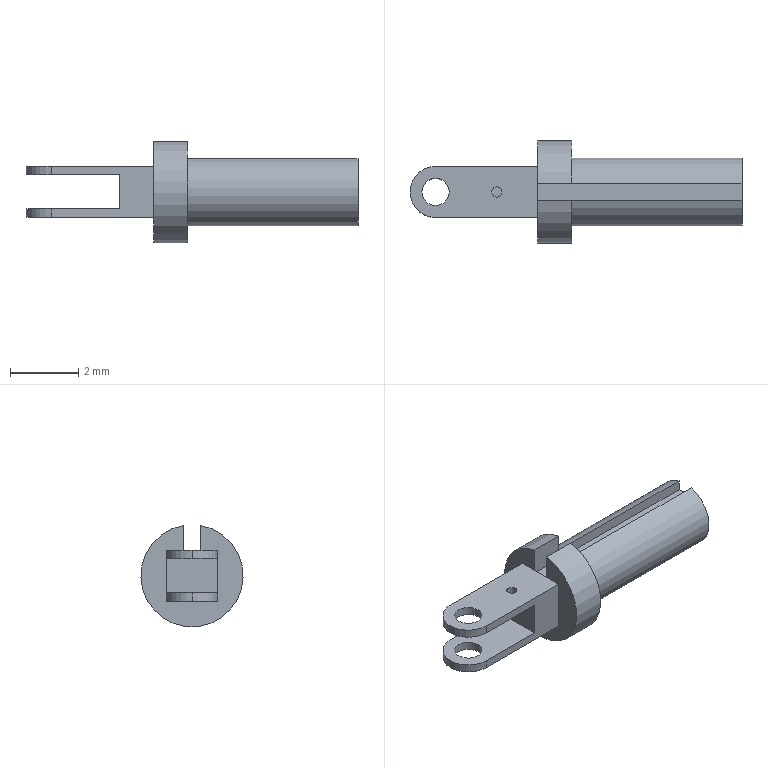Part | SolidWorks | features ICE 5, Revolution 1 | 1 solid | 29 faces | box 9.75 x 3 x 2.979 mm | volume 20.717 mm3 | plane 15 | cylinder 14 | commonest cylinder face diameters 0.8 x4 1.5 x4 0.3 x2 1 x2 2 x1 3 x1
STEP:
#1=CARTESIAN_POINT('',(-1.05,0.,0.5));
#2=VERTEX_POINT('',#1);
#3=CARTESIAN_POINT('',(-1.35,0.,0.5));
#4=VERTEX_POINT('',#3);
#5=CARTESIAN_POINT('',(-1.2,0.,0.5));
#6=DIRECTION('',(0.,0.,-1.));
#7=DIRECTION('',(-1.,0.,0.));
#8=AXIS2_PLACEMENT_3D('',#5,#6,#7);
#9=CIRCLE('',#8,0.15);
#10=EDGE_CURVE('',#2,#4,#9,.T.);
#11=ORIENTED_EDGE('',*,*,#10,.T.);
#12=CARTESIAN_POINT('',(-1.35,0.,0.75));
#13=VERTEX_POINT('',#12);
#14=CARTESIAN_POINT('',(-1.35,0.,-0.25));
#15=DIRECTION('',(0.,0.,1.));
#16=VECTOR('',#15,1000.);
#17=LINE('',#14,#16);
#18=EDGE_CURVE('',#4,#13,#17,.T.);
#19=ORIENTED_EDGE('',*,*,#18,.T.);
#20=CARTESIAN_POINT('',(-1.05,0.,0.75));
#21=VERTEX_POINT('',#20);
#22=CARTESIAN_POINT('',(-1.2,0.,0.75));
#23=DIRECTION('',(0.,0.,1.));
#24=DIRECTION('',(1.,0.,0.));
#25=AXIS2_PLACEMENT_3D('',#22,#23,#24);
#26=CIRCLE('',#25,0.15);
#27=EDGE_CURVE('',#13,#21,#26,.T.);
#28=ORIENTED_EDGE('',*,*,#27,.T.);
#29=CARTESIAN_POINT('',(-1.05,0.,-0.25));
#30=DIRECTION('',(0.,0.,1.));
#31=VECTOR('',#30,1000.);
#32=LINE('',#29,#31);
#33=EDGE_CURVE('',#2,#21,#32,.T.);
#34=ORIENTED_EDGE('',*,*,#33,.F.);
#35=EDGE_LOOP('',(#11,#19,#28,#34));
#36=FACE_OUTER_BOUND('',#35,.T.);
#37=CARTESIAN_POINT('',(-1.2,0.,-0.25));
#38=DIRECTION('',(0.,0.,1.));
#39=DIRECTION('',(1.,0.,0.));
#40=AXIS2_PLACEMENT_3D('',#37,#38,#39);
#41=CYLINDRICAL_SURFACE('',#40,0.15);
#42=ADVANCED_FACE('',(#36),#41,.F.);
#43=CARTESIAN_POINT('',(0.,0.,0.5));
#44=VERTEX_POINT('',#43);
#45=CARTESIAN_POINT('',(0.,0.,-0.5));
#46=VERTEX_POINT('',#45);
#47=CARTESIAN_POINT('',(0.,0.,0.));
#48=DIRECTION('',(1.,0.,0.));
#49=DIRECTION('',(0.,0.,-1.));
#50=AXIS2_PLACEMENT_3D('',#47,#48,#49);
#51=CIRCLE('',#50,0.5);
#52=EDGE_CURVE('',#44,#46,#51,.T.);
#53=ORIENTED_EDGE('',*,*,#52,.F.);
#54=CARTESIAN_POINT('',(6.,0.,0.5));
#55=VERTEX_POINT('',#54);
#56=CARTESIAN_POINT('',(0.,0.,0.5));
#57=DIRECTION('',(1.,0.,0.));
#58=VECTOR('',#57,1000.);
#59=LINE('',#56,#58);
#60=EDGE_CURVE('',#44,#55,#59,.T.);
#61=ORIENTED_EDGE('',*,*,#60,.T.);
#62=CARTESIAN_POINT('',(6.,0.,-0.5));
#63=VERTEX_POINT('',#62);
#64=CARTESIAN_POINT('',(6.,0.,0.));
#65=DIRECTION('',(1.,0.,0.));
#66=DIRECTION('',(0.,0.,-1.));
#67=AXIS2_PLACEMENT_3D('',#64,#65,#66);
#68=CIRCLE('',#67,0.5);
#69=EDGE_CURVE('',#55,#63,#68,.T.);
#70=ORIENTED_EDGE('',*,*,#69,.T.);
#71=CARTESIAN_POINT('',(0.,0.,-0.5));
#72=DIRECTION('',(1.,0.,0.));
#73=VECTOR('',#72,1000.);
#74=LINE('',#71,#73);
#75=EDGE_CURVE('',#46,#63,#74,.T.);
#76=ORIENTED_EDGE('',*,*,#75,.F.);
#77=EDGE_LOOP('',(#53,#61,#70,#76));
#78=FACE_OUTER_BOUND('',#77,.T.);
#79=CARTESIAN_POINT('',(0.,0.,0.));
#80=DIRECTION('',(1.,0.,0.));
#81=DIRECTION('',(0.,0.,-1.));
#82=AXIS2_PLACEMENT_3D('',#79,#80,#81);
#83=CYLINDRICAL_SURFACE('',#82,0.5);
#84=ADVANCED_FACE('',(#78),#83,.F.);
#85=CARTESIAN_POINT('',(-2.6,0.,-0.5));
#86=VERTEX_POINT('',#85);
#87=CARTESIAN_POINT('',(-3.4,0.,-0.5));
#88=VERTEX_POINT('',#87);
#89=CARTESIAN_POINT('',(-3.,0.,-0.5));
#90=DIRECTION('',(0.,0.,-1.));
#91=DIRECTION('',(-1.,0.,0.));
#92=AXIS2_PLACEMENT_3D('',#89,#90,#91);
#93=CIRCLE('',#92,0.4);
#94=EDGE_CURVE('',#86,#88,#93,.T.);
#95=ORIENTED_EDGE('',*,*,#94,.F.);
#96=CARTESIAN_POINT('',(-2.6,0.,-0.75));
#97=VERTEX_POINT('',#96);
#98=CARTESIAN_POINT('',(-2.6,0.,0.75));
#99=DIRECTION('',(0.,0.,-1.));
#100=VECTOR('',#99,1000.);
#101=LINE('',#98,#100);
#102=EDGE_CURVE('',#86,#97,#101,.T.);
#103=ORIENTED_EDGE('',*,*,#102,.T.);
#104=CARTESIAN_POINT('',(-3.4,0.,-0.75));
#105=VERTEX_POINT('',#104);
#106=CARTESIAN_POINT('',(-3.,0.,-0.75));
#107=DIRECTION('',(0.,0.,1.));
#108=DIRECTION('',(1.,0.,0.));
#109=AXIS2_PLACEMENT_3D('',#106,#107,#108);
#110=CIRCLE('',#109,0.4);
#111=EDGE_CURVE('',#105,#97,#110,.T.);
#112=ORIENTED_EDGE('',*,*,#111,.F.);
#113=CARTESIAN_POINT('',(-3.4,0.,0.75));
#114=DIRECTION('',(0.,0.,-1.));
#115=VECTOR('',#114,1000.);
#116=LINE('',#113,#115);
#117=EDGE_CURVE('',#88,#105,#116,.T.);
#118=ORIENTED_EDGE('',*,*,#117,.F.);
#119=EDGE_LOOP('',(#95,#103,#112,#118));
#120=FACE_OUTER_BOUND('',#119,.T.);
#121=CARTESIAN_POINT('',(-3.,0.,0.75));
#122=DIRECTION('',(0.,0.,-1.));
#123=DIRECTION('',(-1.,0.,0.));
#124=AXIS2_PLACEMENT_3D('',#121,#122,#123);
#125=CYLINDRICAL_SURFACE('',#124,0.4);
#126=ADVANCED_FACE('',(#120),#125,.F.);
#127=CARTESIAN_POINT('',(-3.75,0.,-0.5));
#128=VERTEX_POINT('',#127);
#129=CARTESIAN_POINT('',(-3.,-0.75,-0.5));
#130=VERTEX_POINT('',#129);
#131=CARTESIAN_POINT('',(-3.,0.,-0.5));
#132=DIRECTION('',(0.,0.,1.));
#133=DIRECTION('',(-1.,0.,0.));
#134=AXIS2_PLACEMENT_3D('',#131,#132,#133);
#135=CIRCLE('',#134,0.75);
#136=EDGE_CURVE('',#128,#130,#135,.T.);
#137=ORIENTED_EDGE('',*,*,#136,.F.);
#138=CARTESIAN_POINT('',(-3.75,0.,-0.75));
#139=VERTEX_POINT('',#138);
#140=CARTESIAN_POINT('',(-3.75,0.,0.75));
#141=DIRECTION('',(0.,0.,-1.));
#142=VECTOR('',#141,1000.);
#143=LINE('',#140,#142);
#144=EDGE_CURVE('',#128,#139,#143,.T.);
#145=ORIENTED_EDGE('',*,*,#144,.T.);
#146=CARTESIAN_POINT('',(-3.,-0.75,-0.75));
#147=VERTEX_POINT('',#146);
#148=CARTESIAN_POINT('',(-3.,0.,-0.75));
#149=DIRECTION('',(0.,0.,1.));
#150=DIRECTION('',(-1.,0.,0.));
#151=AXIS2_PLACEMENT_3D('',#148,#149,#150);
#152=CIRCLE('',#151,0.75);
#153=EDGE_CURVE('',#139,#147,#152,.T.);
#154=ORIENTED_EDGE('',*,*,#153,.T.);
#155=CARTESIAN_POINT('',(-3.,-0.75,0.75));
#156=DIRECTION('',(0.,0.,-1.));
#157=VECTOR('',#156,1000.);
#158=LINE('',#155,#157);
#159=EDGE_CURVE('',#130,#147,#158,.T.);
#160=ORIENTED_EDGE('',*,*,#159,.F.);
#161=EDGE_LOOP('',(#137,#145,#154,#160));
#162=FACE_OUTER_BOUND('',#161,.T.);
#163=CARTESIAN_POINT('',(-3.,0.,0.75));
#164=DIRECTION('',(0.,0.,-1.));
#165=DIRECTION('',(-1.,0.,0.));
#166=AXIS2_PLACEMENT_3D('',#163,#164,#165);
#167=CYLINDRICAL_SURFACE('',#166,0.75);
#168=ADVANCED_FACE('',(#162),#167,.T.);
#169=CARTESIAN_POINT('',(-3.4,0.,0.75));
#170=VERTEX_POINT('',#169);
#171=CARTESIAN_POINT('',(-2.6,0.,0.75));
#172=VERTEX_POINT('',#171);
#173=CARTESIAN_POINT('',(-3.,0.,0.75));
#174=DIRECTION('',(0.,0.,1.));
#175=DIRECTION('',(1.,0.,0.));
#176=AXIS2_PLACEMENT_3D('',#173,#174,#175);
#177=CIRCLE('',#176,0.4);
#178=EDGE_CURVE('',#170,#172,#177,.T.);
#179=ORIENTED_EDGE('',*,*,#178,.T.);
#180=CARTESIAN_POINT('',(-2.6,0.,0.5));
#181=VERTEX_POINT('',#180);
#182=CARTESIAN_POINT('',(-2.6,0.,0.75));
#183=DIRECTION('',(0.,0.,-1.));
#184=VECTOR('',#183,1000.);
#185=LINE('',#182,#184);
#186=EDGE_CURVE('',#172,#181,#185,.T.);
#187=ORIENTED_EDGE('',*,*,#186,.T.);
#188=CARTESIAN_POINT('',(-3.4,0.,0.5));
#189=VERTEX_POINT('',#188);
#190=CARTESIAN_POINT('',(-3.,0.,0.5));
#191=DIRECTION('',(0.,0.,-1.));
#192=DIRECTION('',(-1.,0.,0.));
#193=AXIS2_PLACEMENT_3D('',#190,#191,#192);
#194=CIRCLE('',#193,0.4);
#195=EDGE_CURVE('',#181,#189,#194,.T.);
#196=ORIENTED_EDGE('',*,*,#195,.T.);
#197=CARTESIAN_POINT('',(-3.4,0.,0.75));
#198=DIRECTION('',(0.,0.,-1.));
#199=VECTOR('',#198,1000.);
#200=LINE('',#197,#199);
#201=EDGE_CURVE('',#170,#189,#200,.T.);
#202=ORIENTED_EDGE('',*,*,#201,.F.);
#203=EDGE_LOOP('',(#179,#187,#196,#202));
#204=FACE_OUTER_BOUND('',#203,.T.);
#205=CARTESIAN_POINT('',(-3.,0.,0.75));
#206=DIRECTION('',(0.,0.,-1.));
#207=DIRECTION('',(-1.,0.,0.));
#208=AXIS2_PLACEMENT_3D('',#205,#206,#207);
#209=CYLINDRICAL_SURFACE('',#208,0.4);
#210=ADVANCED_FACE('',(#204),#209,.F.);
#211=CARTESIAN_POINT('',(-3.75,0.,0.75));
#212=VERTEX_POINT('',#211);
#213=CARTESIAN_POINT('',(-3.,-0.75,0.75));
#214=VERTEX_POINT('',#213);
#215=CARTESIAN_POINT('',(-3.,0.,0.75));
#216=DIRECTION('',(0.,0.,1.));
#217=DIRECTION('',(-1.,0.,0.));
#218=AXIS2_PLACEMENT_3D('',#215,#216,#217);
#219=CIRCLE('',#218,0.75);
#220=EDGE_CURVE('',#212,#214,#219,.T.);
#221=ORIENTED_EDGE('',*,*,#220,.F.);
#222=CARTESIAN_POINT('',(-3.75,0.,0.5));
#223=VERTEX_POINT('',#222);
#224=CARTESIAN_POINT('',(-3.75,0.,0.75));
#225=DIRECTION('',(0.,0.,-1.));
#226=VECTOR('',#225,1000.);
#227=LINE('',#224,#226);
#228=EDGE_CURVE('',#212,#223,#227,.T.);
#229=ORIENTED_EDGE('',*,*,#228,.T.);
#230=CARTESIAN_POINT('',(-3.,-0.75,0.5));
#231=VERTEX_POINT('',#230);
#232=CARTESIAN_POINT('',(-3.,0.,0.5));
#233=DIRECTION('',(0.,0.,1.));
#234=DIRECTION('',(-1.,0.,0.));
#235=AXIS2_PLACEMENT_3D('',#232,#233,#234);
#236=CIRCLE('',#235,0.75);
#237=EDGE_CURVE('',#223,#231,#236,.T.);
#238=ORIENTED_EDGE('',*,*,#237,.T.);
#239=CARTESIAN_POINT('',(-3.,-0.75,0.75));
#240=DIRECTION('',(0.,0.,-1.));
#241=VECTOR('',#240,1000.);
#242=LINE('',#239,#241);
#243=EDGE_CURVE('',#214,#231,#242,.T.);
#244=ORIENTED_EDGE('',*,*,#243,.F.);
#245=EDGE_LOOP('',(#221,#229,#238,#244));
#246=FACE_OUTER_BOUND('',#245,.T.);
#247=CARTESIAN_POINT('',(-3.,0.,0.75));
#248=DIRECTION('',(0.,0.,-1.));
#249=DIRECTION('',(-1.,0.,0.));
#250=AXIS2_PLACEMENT_3D('',#247,#248,#249);
#251=CYLINDRICAL_SURFACE('',#250,0.75);
#252=ADVANCED_FACE('',(#246),#251,.T.);
#253=CARTESIAN_POINT('',(0.,0.25,1.479));
#254=VERTEX_POINT('',#253);
#255=CARTESIAN_POINT('',(0.,0.25,0.75));
#256=VERTEX_POINT('',#255);
#257=CARTESIAN_POINT('',(0.,0.25,0.));
#258=DIRECTION('',(0.,0.,-1.));
#259=VECTOR('',#258,1000.);
#260=LINE('',#257,#259);
#261=EDGE_CURVE('',#254,#256,#260,.T.);
#262=ORIENTED_EDGE('',*,*,#261,.F.);
#263=CARTESIAN_POINT('',(0.,-0.25,1.479));
#264=VERTEX_POINT('',#263);
#265=CARTESIAN_POINT('',(0.,0.,0.));
#266=DIRECTION('',(-1.,0.,0.));
#267=DIRECTION('',(0.,0.,1.));
#268=AXIS2_PLACEMENT_3D('',#265,#266,#267);
#269=CIRCLE('',#268,1.5);
#270=EDGE_CURVE('',#254,#264,#269,.T.);
#271=ORIENTED_EDGE('',*,*,#270,.T.);
#272=CARTESIAN_POINT('',(0.,-0.25,0.75));
#273=VERTEX_POINT('',#272);
#274=CARTESIAN_POINT('',(0.,-0.25,0.));
#275=DIRECTION('',(0.,0.,-1.));
#276=VECTOR('',#275,1000.);
#277=LINE('',#274,#276);
#278=EDGE_CURVE('',#264,#273,#277,.T.);
#279=ORIENTED_EDGE('',*,*,#278,.T.);
#280=CARTESIAN_POINT('',(0.,-0.75,0.75));
#281=VERTEX_POINT('',#280);
#282=CARTESIAN_POINT('',(0.,0.75,0.75));
#283=DIRECTION('',(0.,1.,0.));
#284=VECTOR('',#283,1000.);
#285=LINE('',#282,#284);
#286=EDGE_CURVE('',#281,#273,#285,.T.);
#287=ORIENTED_EDGE('',*,*,#286,.F.);
#288=CARTESIAN_POINT('',(0.,-0.75,-0.75));
#289=VERTEX_POINT('',#288);
#290=CARTESIAN_POINT('',(0.,-0.75,0.75));
#291=DIRECTION('',(0.,0.,-1.));
#292=VECTOR('',#291,1000.);
#293=LINE('',#290,#292);
#294=EDGE_CURVE('',#281,#289,#293,.T.);
#295=ORIENTED_EDGE('',*,*,#294,.T.);
#296=CARTESIAN_POINT('',(0.,0.75,-0.75));
#297=VERTEX_POINT('',#296);
#298=CARTESIAN_POINT('',(0.,0.75,-0.75));
#299=DIRECTION('',(0.,1.,0.));
#300=VECTOR('',#299,1000.);
#301=LINE('',#298,#300);
#302=EDGE_CURVE('',#289,#297,#301,.T.);
#303=ORIENTED_EDGE('',*,*,#302,.T.);
#304=CARTESIAN_POINT('',(0.,0.75,0.75));
#305=VERTEX_POINT('',#304);
#306=CARTESIAN_POINT('',(0.,0.75,0.75));
#307=DIRECTION('',(0.,0.,-1.));
#308=VECTOR('',#307,1000.);
#309=LINE('',#306,#308);
#310=EDGE_CURVE('',#305,#297,#309,.T.);
#311=ORIENTED_EDGE('',*,*,#310,.F.);
#312=CARTESIAN_POINT('',(0.,0.75,0.75));
#313=DIRECTION('',(0.,1.,0.));
#314=VECTOR('',#313,1000.);
#315=LINE('',#312,#314);
#316=EDGE_CURVE('',#256,#305,#315,.T.);
#317=ORIENTED_EDGE('',*,*,#316,.F.);
#318=EDGE_LOOP('',(#262,#271,#279,#287,#295,#303,#311,#317));
#319=FACE_OUTER_BOUND('',#318,.T.);
#320=CARTESIAN_POINT('',(0.,0.,0.));
#321=DIRECTION('',(1.,0.,0.));
#322=DIRECTION('',(0.,0.,-1.));
#323=AXIS2_PLACEMENT_3D('',#320,#321,#322);
#324=PLANE('',#323);
#325=ADVANCED_FACE('',(#319),#324,.F.);
#326=CARTESIAN_POINT('',(1.,0.25,1.479));
#327=VERTEX_POINT('',#326);
#328=CARTESIAN_POINT('',(0.1244,0.25,1.479));
#329=DIRECTION('',(-1.,0.,0.));
#330=VECTOR('',#329,1000.);
#331=LINE('',#328,#330);
#332=EDGE_CURVE('',#327,#254,#331,.T.);
#333=ORIENTED_EDGE('',*,*,#332,.F.);
#334=CARTESIAN_POINT('',(1.,-0.25,1.479));
#335=VERTEX_POINT('',#334);
#336=CARTESIAN_POINT('',(1.,0.,0.));
#337=DIRECTION('',(-1.,0.,0.));
#338=DIRECTION('',(0.,0.,1.));
#339=AXIS2_PLACEMENT_3D('',#336,#337,#338);
#340=CIRCLE('',#339,1.5);
#341=EDGE_CURVE('',#327,#335,#340,.T.);
#342=ORIENTED_EDGE('',*,*,#341,.T.);
#343=CARTESIAN_POINT('',(0.1244,-0.25,1.479));
#344=DIRECTION('',(-1.,0.,0.));
#345=VECTOR('',#344,1000.);
#346=LINE('',#343,#345);
#347=EDGE_CURVE('',#335,#264,#346,.T.);
#348=ORIENTED_EDGE('',*,*,#347,.T.);
#349=ORIENTED_EDGE('',*,*,#270,.F.);
#350=EDGE_LOOP('',(#333,#342,#348,#349));
#351=FACE_OUTER_BOUND('',#350,.T.);
#352=CARTESIAN_POINT('',(0.1244,0.,0.));
#353=DIRECTION('',(-1.,0.,0.));
#354=DIRECTION('',(0.,0.,1.));
#355=AXIS2_PLACEMENT_3D('',#352,#353,#354);
#356=CYLINDRICAL_SURFACE('',#355,1.5);
#357=ADVANCED_FACE('',(#351),#356,.T.);
#358=CARTESIAN_POINT('',(1.,0.25,0.9682));
#359=VERTEX_POINT('',#358);
#360=CARTESIAN_POINT('',(1.,0.25,0.));
#361=DIRECTION('',(0.,0.,1.));
#362=VECTOR('',#361,1000.);
#363=LINE('',#360,#362);
#364=EDGE_CURVE('',#359,#327,#363,.T.);
#365=ORIENTED_EDGE('',*,*,#364,.F.);
#366=CARTESIAN_POINT('',(1.,-0.25,0.9682));
#367=VERTEX_POINT('',#366);
#368=CARTESIAN_POINT('',(1.,0.,0.));
#369=DIRECTION('',(-1.,0.,0.));
#370=DIRECTION('',(0.,0.,1.));
#371=AXIS2_PLACEMENT_3D('',#368,#369,#370);
#372=CIRCLE('',#371,1.);
#373=EDGE_CURVE('',#359,#367,#372,.T.);
#374=ORIENTED_EDGE('',*,*,#373,.T.);
#375=CARTESIAN_POINT('',(1.,-0.25,0.));
#376=DIRECTION('',(0.,0.,1.));
#377=VECTOR('',#376,1000.);
#378=LINE('',#375,#377);
#379=EDGE_CURVE('',#367,#335,#378,.T.);
#380=ORIENTED_EDGE('',*,*,#379,.T.);
#381=ORIENTED_EDGE('',*,*,#341,.F.);
#382=EDGE_LOOP('',(#365,#374,#380,#381));
#383=FACE_OUTER_BOUND('',#382,.T.);
#384=CARTESIAN_POINT('',(1.,1.5,0.));
#385=DIRECTION('',(-1.,0.,0.));
#386=DIRECTION('',(0.,0.,1.));
#387=AXIS2_PLACEMENT_3D('',#384,#385,#386);
#388=PLANE('',#387);
#389=ADVANCED_FACE('',(#383),#388,.F.);
#390=CARTESIAN_POINT('',(6.,0.25,0.9682));
#391=VERTEX_POINT('',#390);
#392=CARTESIAN_POINT('',(0.1244,0.25,0.9682));
#393=DIRECTION('',(-1.,0.,0.));
#394=VECTOR('',#393,1000.);
#395=LINE('',#392,#394);
#396=EDGE_CURVE('',#391,#359,#395,.T.);
#397=ORIENTED_EDGE('',*,*,#396,.F.);
#398=CARTESIAN_POINT('',(6.,-0.25,0.9682));
#399=VERTEX_POINT('',#398);
#400=CARTESIAN_POINT('',(6.,0.,0.));
#401=DIRECTION('',(-1.,0.,0.));
#402=DIRECTION('',(0.,0.,1.));
#403=AXIS2_PLACEMENT_3D('',#400,#401,#402);
#404=CIRCLE('',#403,1.);
#405=EDGE_CURVE('',#391,#399,#404,.T.);
#406=ORIENTED_EDGE('',*,*,#405,.T.);
#407=CARTESIAN_POINT('',(0.1244,-0.25,0.9682));
#408=DIRECTION('',(-1.,0.,0.));
#409=VECTOR('',#408,1000.);
#410=LINE('',#407,#409);
#411=EDGE_CURVE('',#399,#367,#410,.T.);
#412=ORIENTED_EDGE('',*,*,#411,.T.);
#413=ORIENTED_EDGE('',*,*,#373,.F.);
#414=EDGE_LOOP('',(#397,#406,#412,#413));
#415=FACE_OUTER_BOUND('',#414,.T.);
#416=CARTESIAN_POINT('',(0.1244,0.,0.));
#417=DIRECTION('',(-1.,0.,0.));
#418=DIRECTION('',(0.,0.,1.));
#419=AXIS2_PLACEMENT_3D('',#416,#417,#418);
#420=CYLINDRICAL_SURFACE('',#419,1.);
#421=ADVANCED_FACE('',(#415),#420,.T.);
#422=CARTESIAN_POINT('',(6.,0.,0.));
#423=DIRECTION('',(1.,0.,0.));
#424=DIRECTION('',(0.,0.,-1.));
#425=AXIS2_PLACEMENT_3D('',#422,#423,#424);
#426=CIRCLE('',#425,0.5);
#427=EDGE_CURVE('',#63,#55,#426,.T.);
#428=ORIENTED_EDGE('',*,*,#427,.F.);
#429=ORIENTED_EDGE('',*,*,#69,.F.);
#430=EDGE_LOOP('',(#428,#429));
#431=FACE_BOUND('',#430,.T.);
#432=CARTESIAN_POINT('',(6.,0.25,0.65));
#433=VERTEX_POINT('',#432);
#434=CARTESIAN_POINT('',(6.,0.25,0.));
#435=DIRECTION('',(0.,0.,1.));
#436=VECTOR('',#435,1000.);
#437=LINE('',#434,#436);
#438=EDGE_CURVE('',#433,#391,#437,.T.);
#439=ORIENTED_EDGE('',*,*,#438,.F.);
#440=CARTESIAN_POINT('',(6.,-0.25,0.65));
#441=VERTEX_POINT('',#440);
#442=CARTESIAN_POINT('',(6.,0.,0.65));
#443=DIRECTION('',(0.,-1.,0.));
#444=VECTOR('',#443,1000.);
#445=LINE('',#442,#444);
#446=EDGE_CURVE('',#433,#441,#445,.T.);
#447=ORIENTED_EDGE('',*,*,#446,.T.);
#448=CARTESIAN_POINT('',(6.,-0.25,0.));
#449=DIRECTION('',(0.,0.,1.));
#450=VECTOR('',#449,1000.);
#451=LINE('',#448,#450);
#452=EDGE_CURVE('',#441,#399,#451,.T.);
#453=ORIENTED_EDGE('',*,*,#452,.T.);
#454=ORIENTED_EDGE('',*,*,#405,.F.);
#455=EDGE_LOOP('',(#439,#447,#453,#454));
#456=FACE_OUTER_BOUND('',#455,.T.);
#457=CARTESIAN_POINT('',(6.,1.,0.));
#458=DIRECTION('',(-1.,0.,0.));
#459=DIRECTION('',(0.,0.,1.));
#460=AXIS2_PLACEMENT_3D('',#457,#458,#459);
#461=PLANE('',#460);
#462=ADVANCED_FACE('',(#431,#456),#461,.F.);
#463=ORIENTED_EDGE('',*,*,#228,.F.);
#464=CARTESIAN_POINT('',(-3.,0.75,0.75));
#465=VERTEX_POINT('',#464);
#466=CARTESIAN_POINT('',(-3.,0.,0.75));
#467=DIRECTION('',(0.,0.,1.));
#468=DIRECTION('',(-1.,0.,0.));
#469=AXIS2_PLACEMENT_3D('',#466,#467,#468);
#470=CIRCLE('',#469,0.75);
#471=EDGE_CURVE('',#465,#212,#470,.T.);
#472=ORIENTED_EDGE('',*,*,#471,.F.);
#473=CARTESIAN_POINT('',(-3.,0.75,0.5));
#474=VERTEX_POINT('',#473);
#475=CARTESIAN_POINT('',(-3.,0.75,0.75));
#476=DIRECTION('',(0.,0.,-1.));
#477=VECTOR('',#476,1000.);
#478=LINE('',#475,#477);
#479=EDGE_CURVE('',#465,#474,#478,.T.);
#480=ORIENTED_EDGE('',*,*,#479,.T.);
#481=CARTESIAN_POINT('',(-3.,0.,0.5));
#482=DIRECTION('',(0.,0.,1.));
#483=DIRECTION('',(-1.,0.,0.));
#484=AXIS2_PLACEMENT_3D('',#481,#482,#483);
#485=CIRCLE('',#484,0.75);
#486=EDGE_CURVE('',#474,#223,#485,.T.);
#487=ORIENTED_EDGE('',*,*,#486,.T.);
#488=EDGE_LOOP('',(#463,#472,#480,#487));
#489=FACE_OUTER_BOUND('',#488,.T.);
#490=CARTESIAN_POINT('',(-3.,0.,0.75));
#491=DIRECTION('',(0.,0.,-1.));
#492=DIRECTION('',(-1.,0.,0.));
#493=AXIS2_PLACEMENT_3D('',#490,#491,#492);
#494=CYLINDRICAL_SURFACE('',#493,0.75);
#495=ADVANCED_FACE('',(#489),#494,.T.);
#496=ORIENTED_EDGE('',*,*,#186,.F.);
#497=CARTESIAN_POINT('',(-3.,0.,0.75));
#498=DIRECTION('',(0.,0.,1.));
#499=DIRECTION('',(1.,0.,0.));
#500=AXIS2_PLACEMENT_3D('',#497,#498,#499);
#501=CIRCLE('',#500,0.4);
#502=EDGE_CURVE('',#172,#170,#501,.T.);
#503=ORIENTED_EDGE('',*,*,#502,.T.);
#504=ORIENTED_EDGE('',*,*,#201,.T.);
#505=CARTESIAN_POINT('',(-3.,0.,0.5));
#506=DIRECTION('',(0.,0.,-1.));
#507=DIRECTION('',(-1.,0.,0.));
#508=AXIS2_PLACEMENT_3D('',#505,#506,#507);
#509=CIRCLE('',#508,0.4);
#510=EDGE_CURVE('',#189,#181,#509,.T.);
#511=ORIENTED_EDGE('',*,*,#510,.T.);
#512=EDGE_LOOP('',(#496,#503,#504,#511));
#513=FACE_OUTER_BOUND('',#512,.T.);
#514=CARTESIAN_POINT('',(-3.,0.,0.75));
#515=DIRECTION('',(0.,0.,-1.));
#516=DIRECTION('',(-1.,0.,0.));
#517=AXIS2_PLACEMENT_3D('',#514,#515,#516);
#518=CYLINDRICAL_SURFACE('',#517,0.4);
#519=ADVANCED_FACE('',(#513),#518,.F.);
#520=CARTESIAN_POINT('',(-1.2,0.,0.75));
#521=DIRECTION('',(0.,0.,1.));
#522=DIRECTION('',(1.,0.,0.));
#523=AXIS2_PLACEMENT_3D('',#520,#521,#522);
#524=CIRCLE('',#523,0.15);
#525=EDGE_CURVE('',#21,#13,#524,.T.);
#526=ORIENTED_EDGE('',*,*,#525,.F.);
#527=ORIENTED_EDGE('',*,*,#27,.F.);
#528=EDGE_LOOP('',(#526,#527));
#529=FACE_BOUND('',#528,.T.);
#530=CARTESIAN_POINT('',(0.,-0.75,0.75));
#531=DIRECTION('',(1.,0.,0.));
#532=VECTOR('',#531,1000.);
#533=LINE('',#530,#532);
#534=EDGE_CURVE('',#214,#281,#533,.T.);
#535=ORIENTED_EDGE('',*,*,#534,.T.);
#536=ORIENTED_EDGE('',*,*,#286,.T.);
#537=CARTESIAN_POINT('',(0.,0.75,0.75));
#538=DIRECTION('',(0.,1.,0.));
#539=VECTOR('',#538,1000.);
#540=LINE('',#537,#539);
#541=EDGE_CURVE('',#273,#256,#540,.T.);
#542=ORIENTED_EDGE('',*,*,#541,.T.);
#543=ORIENTED_EDGE('',*,*,#316,.T.);
#544=CARTESIAN_POINT('',(0.,0.75,0.75));
#545=DIRECTION('',(-1.,0.,0.));
#546=VECTOR('',#545,1000.);
#547=LINE('',#544,#546);
#548=EDGE_CURVE('',#305,#465,#547,.T.);
#549=ORIENTED_EDGE('',*,*,#548,.T.);
#550=ORIENTED_EDGE('',*,*,#471,.T.);
#551=ORIENTED_EDGE('',*,*,#220,.T.);
#552=EDGE_LOOP('',(#535,#536,#542,#543,#549,#550,#551));
#553=FACE_OUTER_BOUND('',#552,.T.);
#554=ORIENTED_EDGE('',*,*,#178,.F.);
#555=ORIENTED_EDGE('',*,*,#502,.F.);
#556=EDGE_LOOP('',(#554,#555));
#557=FACE_BOUND('',#556,.T.);
#558=CARTESIAN_POINT('',(-3.,0.,0.75));
#559=DIRECTION('',(0.,0.,-1.));
#560=DIRECTION('',(-1.,0.,0.));
#561=AXIS2_PLACEMENT_3D('',#558,#559,#560);
#562=PLANE('',#561);
#563=ADVANCED_FACE('',(#529,#553,#557),#562,.F.);
#564=CARTESIAN_POINT('',(0.,-0.75,-0.75));
#565=DIRECTION('',(1.,0.,0.));
#566=VECTOR('',#565,1000.);
#567=LINE('',#564,#566);
#568=EDGE_CURVE('',#147,#289,#567,.T.);
#569=ORIENTED_EDGE('',*,*,#568,.F.);
#570=ORIENTED_EDGE('',*,*,#153,.F.);
#571=CARTESIAN_POINT('',(-3.,0.75,-0.75));
#572=VERTEX_POINT('',#571);
#573=CARTESIAN_POINT('',(-3.,0.,-0.75));
#574=DIRECTION('',(0.,0.,1.));
#575=DIRECTION('',(-1.,0.,0.));
#576=AXIS2_PLACEMENT_3D('',#573,#574,#575);
#577=CIRCLE('',#576,0.75);
#578=EDGE_CURVE('',#572,#139,#577,.T.);
#579=ORIENTED_EDGE('',*,*,#578,.F.);
#580=CARTESIAN_POINT('',(0.,0.75,-0.75));
#581=DIRECTION('',(-1.,0.,0.));
#582=VECTOR('',#581,1000.);
#583=LINE('',#580,#582);
#584=EDGE_CURVE('',#297,#572,#583,.T.);
#585=ORIENTED_EDGE('',*,*,#584,.F.);
#586=ORIENTED_EDGE('',*,*,#302,.F.);
#587=EDGE_LOOP('',(#569,#570,#579,#585,#586));
#588=FACE_OUTER_BOUND('',#587,.T.);
#589=ORIENTED_EDGE('',*,*,#111,.T.);
#590=CARTESIAN_POINT('',(-3.,0.,-0.75));
#591=DIRECTION('',(0.,0.,1.));
#592=DIRECTION('',(1.,0.,0.));
#593=AXIS2_PLACEMENT_3D('',#590,#591,#592);
#594=CIRCLE('',#593,0.4);
#595=EDGE_CURVE('',#97,#105,#594,.T.);
#596=ORIENTED_EDGE('',*,*,#595,.T.);
#597=EDGE_LOOP('',(#589,#596));
#598=FACE_BOUND('',#597,.T.);
#599=CARTESIAN_POINT('',(-3.,0.,-0.75));
#600=DIRECTION('',(0.,0.,-1.));
#601=DIRECTION('',(-1.,0.,0.));
#602=AXIS2_PLACEMENT_3D('',#599,#600,#601);
#603=PLANE('',#602);
#604=ADVANCED_FACE('',(#588,#598),#603,.T.);
#605=CARTESIAN_POINT('',(-1.,-0.75,-0.5));
#606=VERTEX_POINT('',#605);
#607=CARTESIAN_POINT('',(-1.,-0.75,0.5));
#608=VERTEX_POINT('',#607);
#609=CARTESIAN_POINT('',(-1.,-0.75,-0.5));
#610=DIRECTION('',(0.,0.,1.));
#611=VECTOR('',#610,1000.);
#612=LINE('',#609,#611);
#613=EDGE_CURVE('',#606,#608,#612,.T.);
#614=ORIENTED_EDGE('',*,*,#613,.F.);
#615=CARTESIAN_POINT('',(-1.,-0.75,-0.5));
#616=DIRECTION('',(1.,0.,0.));
#617=VECTOR('',#616,1000.);
#618=LINE('',#615,#617);
#619=EDGE_CURVE('',#130,#606,#618,.T.);
#620=ORIENTED_EDGE('',*,*,#619,.F.);
#621=ORIENTED_EDGE('',*,*,#159,.T.);
#622=ORIENTED_EDGE('',*,*,#568,.T.);
#623=ORIENTED_EDGE('',*,*,#294,.F.);
#624=ORIENTED_EDGE('',*,*,#534,.F.);
#625=ORIENTED_EDGE('',*,*,#243,.T.);
#626=CARTESIAN_POINT('',(-1.,-0.75,0.5));
#627=DIRECTION('',(1.,0.,0.));
#628=VECTOR('',#627,1000.);
#629=LINE('',#626,#628);
#630=EDGE_CURVE('',#231,#608,#629,.T.);
#631=ORIENTED_EDGE('',*,*,#630,.T.);
#632=EDGE_LOOP('',(#614,#620,#621,#622,#623,#624,#625,#631));
#633=FACE_OUTER_BOUND('',#632,.T.);
#634=CARTESIAN_POINT('',(0.,-0.75,0.75));
#635=DIRECTION('',(0.,1.,0.));
#636=DIRECTION('',(-1.,0.,0.));
#637=AXIS2_PLACEMENT_3D('',#634,#635,#636);
#638=PLANE('',#637);
#639=ADVANCED_FACE('',(#633),#638,.F.);
#640=CARTESIAN_POINT('',(-3.,0.75,-0.5));
#641=VERTEX_POINT('',#640);
#642=CARTESIAN_POINT('',(-3.,0.75,0.75));
#643=DIRECTION('',(0.,0.,-1.));
#644=VECTOR('',#643,1000.);
#645=LINE('',#642,#644);
#646=EDGE_CURVE('',#641,#572,#645,.T.);
#647=ORIENTED_EDGE('',*,*,#646,.F.);
#648=CARTESIAN_POINT('',(-1.,0.75,-0.5));
#649=VERTEX_POINT('',#648);
#650=CARTESIAN_POINT('',(-3.,0.75,-0.5));
#651=DIRECTION('',(-1.,0.,0.));
#652=VECTOR('',#651,1000.);
#653=LINE('',#650,#652);
#654=EDGE_CURVE('',#649,#641,#653,.T.);
#655=ORIENTED_EDGE('',*,*,#654,.F.);
#656=CARTESIAN_POINT('',(-1.,0.75,0.5));
#657=VERTEX_POINT('',#656);
#658=CARTESIAN_POINT('',(-1.,0.75,-0.5));
#659=DIRECTION('',(0.,0.,1.));
#660=VECTOR('',#659,1000.);
#661=LINE('',#658,#660);
#662=EDGE_CURVE('',#649,#657,#661,.T.);
#663=ORIENTED_EDGE('',*,*,#662,.T.);
#664=CARTESIAN_POINT('',(-3.,0.75,0.5));
#665=DIRECTION('',(-1.,0.,0.));
#666=VECTOR('',#665,1000.);
#667=LINE('',#664,#666);
#668=EDGE_CURVE('',#657,#474,#667,.T.);
#669=ORIENTED_EDGE('',*,*,#668,.T.);
#670=ORIENTED_EDGE('',*,*,#479,.F.);
#671=ORIENTED_EDGE('',*,*,#548,.F.);
#672=ORIENTED_EDGE('',*,*,#310,.T.);
#673=ORIENTED_EDGE('',*,*,#584,.T.);
#674=EDGE_LOOP('',(#647,#655,#663,#669,#670,#671,#672,#673));
#675=FACE_OUTER_BOUND('',#674,.T.);
#676=CARTESIAN_POINT('',(0.,0.75,0.75));
#677=DIRECTION('',(0.,-1.,0.));
#678=DIRECTION('',(1.,0.,0.));
#679=AXIS2_PLACEMENT_3D('',#676,#677,#678);
#680=PLANE('',#679);
#681=ADVANCED_FACE('',(#675),#680,.F.);
#682=ORIENTED_EDGE('',*,*,#144,.F.);
#683=CARTESIAN_POINT('',(-3.,0.,-0.5));
#684=DIRECTION('',(0.,0.,1.));
#685=DIRECTION('',(-1.,0.,0.));
#686=AXIS2_PLACEMENT_3D('',#683,#684,#685);
#687=CIRCLE('',#686,0.75);
#688=EDGE_CURVE('',#641,#128,#687,.T.);
#689=ORIENTED_EDGE('',*,*,#688,.F.);
#690=ORIENTED_EDGE('',*,*,#646,.T.);
#691=ORIENTED_EDGE('',*,*,#578,.T.);
#692=EDGE_LOOP('',(#682,#689,#690,#691));
#693=FACE_OUTER_BOUND('',#692,.T.);
#694=CARTESIAN_POINT('',(-3.,0.,0.75));
#695=DIRECTION('',(0.,0.,-1.));
#696=DIRECTION('',(-1.,0.,0.));
#697=AXIS2_PLACEMENT_3D('',#694,#695,#696);
#698=CYLINDRICAL_SURFACE('',#697,0.75);
#699=ADVANCED_FACE('',(#693),#698,.T.);
#700=ORIENTED_EDGE('',*,*,#102,.F.);
#701=CARTESIAN_POINT('',(-3.,0.,-0.5));
#702=DIRECTION('',(0.,0.,-1.));
#703=DIRECTION('',(-1.,0.,0.));
#704=AXIS2_PLACEMENT_3D('',#701,#702,#703);
#705=CIRCLE('',#704,0.4);
#706=EDGE_CURVE('',#88,#86,#705,.T.);
#707=ORIENTED_EDGE('',*,*,#706,.F.);
#708=ORIENTED_EDGE('',*,*,#117,.T.);
#709=ORIENTED_EDGE('',*,*,#595,.F.);
#710=EDGE_LOOP('',(#700,#707,#708,#709));
#711=FACE_OUTER_BOUND('',#710,.T.);
#712=CARTESIAN_POINT('',(-3.,0.,0.75));
#713=DIRECTION('',(0.,0.,-1.));
#714=DIRECTION('',(-1.,0.,0.));
#715=AXIS2_PLACEMENT_3D('',#712,#713,#714);
#716=CYLINDRICAL_SURFACE('',#715,0.4);
#717=ADVANCED_FACE('',(#711),#716,.F.);
#718=CARTESIAN_POINT('',(-1.,0.75,0.5));
#719=DIRECTION('',(0.,1.,0.));
#720=VECTOR('',#719,1000.);
#721=LINE('',#718,#720);
#722=EDGE_CURVE('',#608,#657,#721,.T.);
#723=ORIENTED_EDGE('',*,*,#722,.T.);
#724=ORIENTED_EDGE('',*,*,#662,.F.);
#725=CARTESIAN_POINT('',(-1.,0.75,-0.5));
#726=DIRECTION('',(0.,1.,0.));
#727=VECTOR('',#726,1000.);
#728=LINE('',#725,#727);
#729=EDGE_CURVE('',#606,#649,#728,.T.);
#730=ORIENTED_EDGE('',*,*,#729,.F.);
#731=ORIENTED_EDGE('',*,*,#613,.T.);
#732=EDGE_LOOP('',(#723,#724,#730,#731));
#733=FACE_OUTER_BOUND('',#732,.T.);
#734=CARTESIAN_POINT('',(-1.,0.75,-0.5));
#735=DIRECTION('',(1.,0.,0.));
#736=DIRECTION('',(0.,0.,-1.));
#737=AXIS2_PLACEMENT_3D('',#734,#735,#736);
#738=PLANE('',#737);
#739=ADVANCED_FACE('',(#733),#738,.F.);
#740=ORIENTED_EDGE('',*,*,#706,.T.);
#741=ORIENTED_EDGE('',*,*,#94,.T.);
#742=EDGE_LOOP('',(#740,#741));
#743=FACE_BOUND('',#742,.T.);
#744=ORIENTED_EDGE('',*,*,#654,.T.);
#745=ORIENTED_EDGE('',*,*,#688,.T.);
#746=ORIENTED_EDGE('',*,*,#136,.T.);
#747=ORIENTED_EDGE('',*,*,#619,.T.);
#748=ORIENTED_EDGE('',*,*,#729,.T.);
#749=EDGE_LOOP('',(#744,#745,#746,#747,#748));
#750=FACE_OUTER_BOUND('',#749,.T.);
#751=CARTESIAN_POINT('',(-3.,0.,-0.5));
#752=DIRECTION('',(0.,0.,-1.));
#753=DIRECTION('',(-1.,0.,0.));
#754=AXIS2_PLACEMENT_3D('',#751,#752,#753);
#755=PLANE('',#754);
#756=ADVANCED_FACE('',(#743,#750),#755,.F.);
#757=ORIENTED_EDGE('',*,*,#10,.F.);
#758=CARTESIAN_POINT('',(-1.2,0.,0.5));
#759=DIRECTION('',(0.,0.,-1.));
#760=DIRECTION('',(-1.,0.,0.));
#761=AXIS2_PLACEMENT_3D('',#758,#759,#760);
#762=CIRCLE('',#761,0.15);
#763=EDGE_CURVE('',#4,#2,#762,.T.);
#764=ORIENTED_EDGE('',*,*,#763,.F.);
#765=EDGE_LOOP('',(#757,#764));
#766=FACE_BOUND('',#765,.T.);
#767=ORIENTED_EDGE('',*,*,#510,.F.);
#768=ORIENTED_EDGE('',*,*,#195,.F.);
#769=EDGE_LOOP('',(#767,#768));
#770=FACE_BOUND('',#769,.T.);
#771=ORIENTED_EDGE('',*,*,#668,.F.);
#772=ORIENTED_EDGE('',*,*,#722,.F.);
#773=ORIENTED_EDGE('',*,*,#630,.F.);
#774=ORIENTED_EDGE('',*,*,#237,.F.);
#775=ORIENTED_EDGE('',*,*,#486,.F.);
#776=EDGE_LOOP('',(#771,#772,#773,#774,#775));
#777=FACE_OUTER_BOUND('',#776,.T.);
#778=CARTESIAN_POINT('',(-3.,0.,0.5));
#779=DIRECTION('',(0.,0.,-1.));
#780=DIRECTION('',(-1.,0.,0.));
#781=AXIS2_PLACEMENT_3D('',#778,#779,#780);
#782=PLANE('',#781);
#783=ADVANCED_FACE('',(#766,#770,#777),#782,.T.);
#784=ORIENTED_EDGE('',*,*,#60,.F.);
#785=CARTESIAN_POINT('',(0.,0.,0.));
#786=DIRECTION('',(1.,0.,0.));
#787=DIRECTION('',(0.,0.,-1.));
#788=AXIS2_PLACEMENT_3D('',#785,#786,#787);
#789=CIRCLE('',#788,0.5);
#790=EDGE_CURVE('',#46,#44,#789,.T.);
#791=ORIENTED_EDGE('',*,*,#790,.F.);
#792=ORIENTED_EDGE('',*,*,#75,.T.);
#793=ORIENTED_EDGE('',*,*,#427,.T.);
#794=EDGE_LOOP('',(#784,#791,#792,#793));
#795=FACE_OUTER_BOUND('',#794,.T.);
#796=CARTESIAN_POINT('',(0.,0.,0.));
#797=DIRECTION('',(1.,0.,0.));
#798=DIRECTION('',(0.,0.,-1.));
#799=AXIS2_PLACEMENT_3D('',#796,#797,#798);
#800=CYLINDRICAL_SURFACE('',#799,0.5);
#801=ADVANCED_FACE('',(#795),#800,.F.);
#802=ORIENTED_EDGE('',*,*,#790,.T.);
#803=ORIENTED_EDGE('',*,*,#52,.T.);
#804=EDGE_LOOP('',(#802,#803));
#805=FACE_OUTER_BOUND('',#804,.T.);
#806=CARTESIAN_POINT('',(0.,0.,0.));
#807=DIRECTION('',(1.,0.,0.));
#808=DIRECTION('',(0.,0.,-1.));
#809=AXIS2_PLACEMENT_3D('',#806,#807,#808);
#810=PLANE('',#809);
#811=ADVANCED_FACE('',(#805),#810,.T.);
#812=ORIENTED_EDGE('',*,*,#332,.T.);
#813=ORIENTED_EDGE('',*,*,#261,.T.);
#814=CARTESIAN_POINT('',(0.,0.25,0.65));
#815=VERTEX_POINT('',#814);
#816=CARTESIAN_POINT('',(0.,0.25,0.));
#817=DIRECTION('',(0.,0.,-1.));
#818=VECTOR('',#817,1000.);
#819=LINE('',#816,#818);
#820=EDGE_CURVE('',#256,#815,#819,.T.);
#821=ORIENTED_EDGE('',*,*,#820,.T.);
#822=CARTESIAN_POINT('',(0.,0.25,0.65));
#823=DIRECTION('',(1.,0.,0.));
#824=VECTOR('',#823,1000.);
#825=LINE('',#822,#824);
#826=EDGE_CURVE('',#815,#433,#825,.T.);
#827=ORIENTED_EDGE('',*,*,#826,.T.);
#828=ORIENTED_EDGE('',*,*,#438,.T.);
#829=ORIENTED_EDGE('',*,*,#396,.T.);
#830=ORIENTED_EDGE('',*,*,#364,.T.);
#831=EDGE_LOOP('',(#812,#813,#821,#827,#828,#829,#830));
#832=FACE_OUTER_BOUND('',#831,.T.);
#833=CARTESIAN_POINT('',(0.,0.25,0.));
#834=DIRECTION('',(0.,-1.,0.));
#835=DIRECTION('',(0.,0.,-1.));
#836=AXIS2_PLACEMENT_3D('',#833,#834,#835);
#837=PLANE('',#836);
#838=ADVANCED_FACE('',(#832),#837,.T.);
#839=ORIENTED_EDGE('',*,*,#379,.F.);
#840=ORIENTED_EDGE('',*,*,#411,.F.);
#841=ORIENTED_EDGE('',*,*,#452,.F.);
#842=CARTESIAN_POINT('',(0.,-0.25,0.65));
#843=VERTEX_POINT('',#842);
#844=CARTESIAN_POINT('',(0.,-0.25,0.65));
#845=DIRECTION('',(1.,0.,0.));
#846=VECTOR('',#845,1000.);
#847=LINE('',#844,#846);
#848=EDGE_CURVE('',#843,#441,#847,.T.);
#849=ORIENTED_EDGE('',*,*,#848,.F.);
#850=CARTESIAN_POINT('',(0.,-0.25,0.));
#851=DIRECTION('',(0.,0.,-1.));
#852=VECTOR('',#851,1000.);
#853=LINE('',#850,#852);
#854=EDGE_CURVE('',#273,#843,#853,.T.);
#855=ORIENTED_EDGE('',*,*,#854,.F.);
#856=ORIENTED_EDGE('',*,*,#278,.F.);
#857=ORIENTED_EDGE('',*,*,#347,.F.);
#858=EDGE_LOOP('',(#839,#840,#841,#849,#855,#856,#857));
#859=FACE_OUTER_BOUND('',#858,.T.);
#860=CARTESIAN_POINT('',(0.,-0.25,0.));
#861=DIRECTION('',(0.,-1.,0.));
#862=DIRECTION('',(0.,0.,-1.));
#863=AXIS2_PLACEMENT_3D('',#860,#861,#862);
#864=PLANE('',#863);
#865=ADVANCED_FACE('',(#859),#864,.F.);
#866=ORIENTED_EDGE('',*,*,#541,.F.);
#867=ORIENTED_EDGE('',*,*,#854,.T.);
#868=CARTESIAN_POINT('',(0.,0.,0.65));
#869=DIRECTION('',(0.,-1.,0.));
#870=VECTOR('',#869,1000.);
#871=LINE('',#868,#870);
#872=EDGE_CURVE('',#815,#843,#871,.T.);
#873=ORIENTED_EDGE('',*,*,#872,.F.);
#874=ORIENTED_EDGE('',*,*,#820,.F.);
#875=EDGE_LOOP('',(#866,#867,#873,#874));
#876=FACE_OUTER_BOUND('',#875,.T.);
#877=CARTESIAN_POINT('',(0.,0.,0.));
#878=DIRECTION('',(1.,0.,0.));
#879=DIRECTION('',(0.,0.,-1.));
#880=AXIS2_PLACEMENT_3D('',#877,#878,#879);
#881=PLANE('',#880);
#882=ADVANCED_FACE('',(#876),#881,.T.);
#883=ORIENTED_EDGE('',*,*,#446,.F.);
#884=ORIENTED_EDGE('',*,*,#826,.F.);
#885=ORIENTED_EDGE('',*,*,#872,.T.);
#886=ORIENTED_EDGE('',*,*,#848,.T.);
#887=EDGE_LOOP('',(#883,#884,#885,#886));
#888=FACE_OUTER_BOUND('',#887,.T.);
#889=CARTESIAN_POINT('',(0.,0.,0.65));
#890=DIRECTION('',(0.,0.,1.));
#891=DIRECTION('',(0.,-1.,0.));
#892=AXIS2_PLACEMENT_3D('',#889,#890,#891);
#893=PLANE('',#892);
#894=ADVANCED_FACE('',(#888),#893,.T.);
#895=ORIENTED_EDGE('',*,*,#18,.F.);
#896=ORIENTED_EDGE('',*,*,#763,.T.);
#897=ORIENTED_EDGE('',*,*,#33,.T.);
#898=ORIENTED_EDGE('',*,*,#525,.T.);
#899=EDGE_LOOP('',(#895,#896,#897,#898));
#900=FACE_OUTER_BOUND('',#899,.T.);
#901=CARTESIAN_POINT('',(-1.2,0.,-0.25));
#902=DIRECTION('',(0.,0.,1.));
#903=DIRECTION('',(1.,0.,0.));
#904=AXIS2_PLACEMENT_3D('',#901,#902,#903);
#905=CYLINDRICAL_SURFACE('',#904,0.15);
#906=ADVANCED_FACE('',(#900),#905,.F.);
#907=CLOSED_SHELL('',(#42,#84,#126,#168,#210,#252,#325,#357,#389,#421,#462,#495,#519,#563,#604,#639,#681,#699,#717,#739,#756,#783,#801,#811,#838,#865,#882,#894,#906));
#908=MANIFOLD_SOLID_BREP('',#907);
#909=CARTESIAN_POINT('',(0.,0.,0.));
#910=DIRECTION('',(0.,0.,1.));
#911=DIRECTION('',(1.,0.,0.));
#912=AXIS2_PLACEMENT_3D('',#909,#910,#911);
#913=(LENGTH_UNIT()NAMED_UNIT(*)SI_UNIT(.MILLI.,.METRE.));
#914=UNCERTAINTY_MEASURE_WITH_UNIT(LENGTH_MEASURE(0.00001),#913,'','');
#915=(NAMED_UNIT(*)PLANE_ANGLE_UNIT()SI_UNIT($,.RADIAN.));
#916=(NAMED_UNIT(*)SI_UNIT($,.STERADIAN.)SOLID_ANGLE_UNIT());
#917=(GEOMETRIC_REPRESENTATION_CONTEXT(3)GLOBAL_UNCERTAINTY_ASSIGNED_CONTEXT((#914))GLOBAL_UNIT_ASSIGNED_CONTEXT((#913,#915,#916))REPRESENTATION_CONTEXT('',''));
#918=ADVANCED_BREP_SHAPE_REPRESENTATION('',(#908,#912),#917);